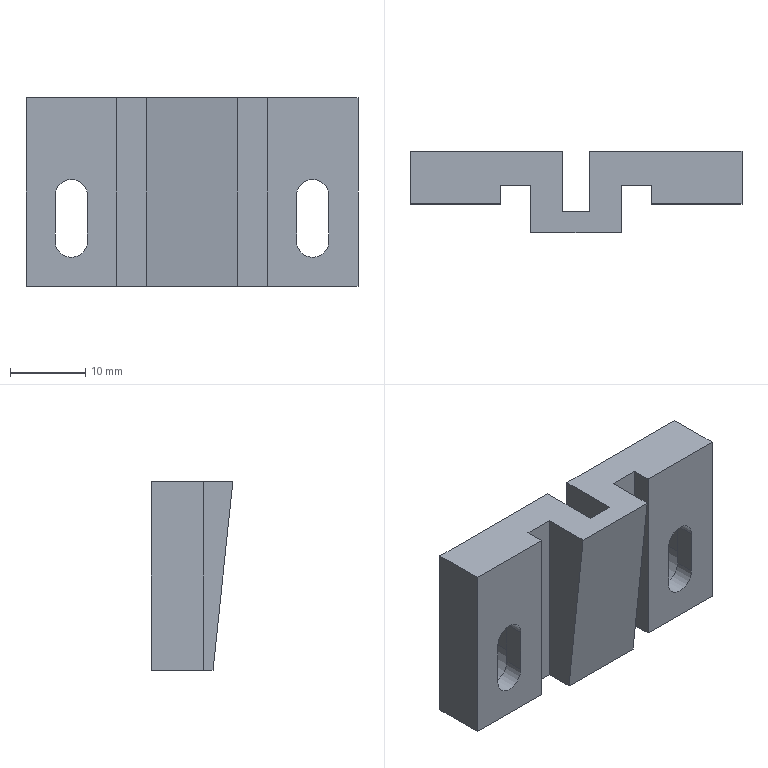Part | NX | features BREP 1 | 1 solid | 40 faces | box 44 x 10.828 x 25 mm | volume 6160 mm3 | plane 28 | cylinder 12 | commonest cylinder face diameters 4.3 x6 8 x6
STEP:
#1=CARTESIAN_POINT('',(16.,-1.,14.15));
#2=VERTEX_POINT('',#1);
#3=CARTESIAN_POINT('',(18.15,-1.,12.));
#4=VERTEX_POINT('',#3);
#5=CARTESIAN_POINT('',(16.,-1.,12.));
#6=DIRECTION('',(0.,1.,0.));
#7=DIRECTION('',(1.,0.,0.));
#8=AXIS2_PLACEMENT_3D('',#5,#6,#7);
#9=CIRCLE('',#8,2.15);
#10=EDGE_CURVE('',#2,#4,#9,.T.);
#11=ORIENTED_EDGE('',*,*,#10,.F.);
#12=CARTESIAN_POINT('',(16.,1.6,14.15));
#13=VERTEX_POINT('',#12);
#14=CARTESIAN_POINT('',(16.,-4.828,14.15));
#15=DIRECTION('',(0.,1.,0.));
#16=VECTOR('',#15,1000.);
#17=LINE('',#14,#16);
#18=EDGE_CURVE('',#2,#13,#17,.T.);
#19=ORIENTED_EDGE('',*,*,#18,.T.);
#20=CARTESIAN_POINT('',(18.15,1.6,12.));
#21=VERTEX_POINT('',#20);
#22=CARTESIAN_POINT('',(16.,1.6,12.));
#23=DIRECTION('',(0.,-1.,0.));
#24=DIRECTION('',(0.,0.,1.));
#25=AXIS2_PLACEMENT_3D('',#22,#23,#24);
#26=CIRCLE('',#25,2.15);
#27=EDGE_CURVE('',#21,#13,#26,.T.);
#28=ORIENTED_EDGE('',*,*,#27,.F.);
#29=CARTESIAN_POINT('',(18.15,-4.828,12.));
#30=DIRECTION('',(0.,1.,0.));
#31=VECTOR('',#30,1000.);
#32=LINE('',#29,#31);
#33=EDGE_CURVE('',#4,#21,#32,.T.);
#34=ORIENTED_EDGE('',*,*,#33,.F.);
#35=EDGE_LOOP('',(#11,#19,#28,#34));
#36=FACE_BOUND('',#35,.T.);
#37=CARTESIAN_POINT('',(16.,-4.828,12.));
#38=DIRECTION('',(0.,1.,0.));
#39=DIRECTION('',(0.,0.,1.));
#40=AXIS2_PLACEMENT_3D('',#37,#38,#39);
#41=CYLINDRICAL_SURFACE('',#40,2.15);
#42=ADVANCED_FACE('',(#36),#41,.F.);
#43=CARTESIAN_POINT('',(20.,1.6,12.));
#44=VERTEX_POINT('',#43);
#45=CARTESIAN_POINT('',(16.,1.6,16.));
#46=VERTEX_POINT('',#45);
#47=CARTESIAN_POINT('',(16.,1.6,12.));
#48=DIRECTION('',(0.,-1.,0.));
#49=DIRECTION('',(0.,0.,-1.));
#50=AXIS2_PLACEMENT_3D('',#47,#48,#49);
#51=CIRCLE('',#50,4.);
#52=EDGE_CURVE('',#44,#46,#51,.T.);
#53=ORIENTED_EDGE('',*,*,#52,.T.);
#54=CARTESIAN_POINT('',(16.,6.,16.));
#55=VERTEX_POINT('',#54);
#56=CARTESIAN_POINT('',(16.,-14.525,16.));
#57=DIRECTION('',(0.,1.,0.));
#58=VECTOR('',#57,1000.);
#59=LINE('',#56,#58);
#60=EDGE_CURVE('',#46,#55,#59,.T.);
#61=ORIENTED_EDGE('',*,*,#60,.T.);
#62=CARTESIAN_POINT('',(20.,6.,12.));
#63=VERTEX_POINT('',#62);
#64=CARTESIAN_POINT('',(16.,6.,12.));
#65=DIRECTION('',(0.,-1.,0.));
#66=DIRECTION('',(0.,0.,1.));
#67=AXIS2_PLACEMENT_3D('',#64,#65,#66);
#68=CIRCLE('',#67,4.);
#69=EDGE_CURVE('',#63,#55,#68,.T.);
#70=ORIENTED_EDGE('',*,*,#69,.F.);
#71=CARTESIAN_POINT('',(20.,-14.525,12.));
#72=DIRECTION('',(0.,1.,0.));
#73=VECTOR('',#72,1000.);
#74=LINE('',#71,#73);
#75=EDGE_CURVE('',#44,#63,#74,.T.);
#76=ORIENTED_EDGE('',*,*,#75,.F.);
#77=EDGE_LOOP('',(#53,#61,#70,#76));
#78=FACE_BOUND('',#77,.T.);
#79=CARTESIAN_POINT('',(16.,-14.525,12.));
#80=DIRECTION('',(0.,1.,0.));
#81=DIRECTION('',(0.,0.,1.));
#82=AXIS2_PLACEMENT_3D('',#79,#80,#81);
#83=CYLINDRICAL_SURFACE('',#82,4.);
#84=ADVANCED_FACE('',(#78),#83,.F.);
#85=CARTESIAN_POINT('',(-16.,-1.,14.15));
#86=VERTEX_POINT('',#85);
#87=CARTESIAN_POINT('',(-13.85,-1.,12.));
#88=VERTEX_POINT('',#87);
#89=CARTESIAN_POINT('',(-16.,-1.,12.));
#90=DIRECTION('',(0.,1.,0.));
#91=DIRECTION('',(-1.,0.,0.));
#92=AXIS2_PLACEMENT_3D('',#89,#90,#91);
#93=CIRCLE('',#92,2.15);
#94=EDGE_CURVE('',#86,#88,#93,.T.);
#95=ORIENTED_EDGE('',*,*,#94,.F.);
#96=CARTESIAN_POINT('',(-16.,1.6,14.15));
#97=VERTEX_POINT('',#96);
#98=CARTESIAN_POINT('',(-16.,-4.828,14.15));
#99=DIRECTION('',(0.,1.,0.));
#100=VECTOR('',#99,1000.);
#101=LINE('',#98,#100);
#102=EDGE_CURVE('',#86,#97,#101,.T.);
#103=ORIENTED_EDGE('',*,*,#102,.T.);
#104=CARTESIAN_POINT('',(-13.85,1.6,12.));
#105=VERTEX_POINT('',#104);
#106=CARTESIAN_POINT('',(-16.,1.6,12.));
#107=DIRECTION('',(0.,1.,0.));
#108=DIRECTION('',(0.,0.,1.));
#109=AXIS2_PLACEMENT_3D('',#106,#107,#108);
#110=CIRCLE('',#109,2.15);
#111=EDGE_CURVE('',#97,#105,#110,.T.);
#112=ORIENTED_EDGE('',*,*,#111,.T.);
#113=CARTESIAN_POINT('',(-13.85,-4.828,12.));
#114=DIRECTION('',(0.,1.,0.));
#115=VECTOR('',#114,1000.);
#116=LINE('',#113,#115);
#117=EDGE_CURVE('',#88,#105,#116,.T.);
#118=ORIENTED_EDGE('',*,*,#117,.F.);
#119=EDGE_LOOP('',(#95,#103,#112,#118));
#120=FACE_BOUND('',#119,.T.);
#121=CARTESIAN_POINT('',(-16.,-4.828,12.));
#122=DIRECTION('',(0.,1.,0.));
#123=DIRECTION('',(0.,0.,1.));
#124=AXIS2_PLACEMENT_3D('',#121,#122,#123);
#125=CYLINDRICAL_SURFACE('',#124,2.15);
#126=ADVANCED_FACE('',(#120),#125,.F.);
#127=CARTESIAN_POINT('',(-16.,1.6,16.));
#128=VERTEX_POINT('',#127);
#129=CARTESIAN_POINT('',(-12.,1.6,12.));
#130=VERTEX_POINT('',#129);
#131=CARTESIAN_POINT('',(-16.,1.6,12.));
#132=DIRECTION('',(0.,1.,0.));
#133=DIRECTION('',(0.,0.,-1.));
#134=AXIS2_PLACEMENT_3D('',#131,#132,#133);
#135=CIRCLE('',#134,4.);
#136=EDGE_CURVE('',#128,#130,#135,.T.);
#137=ORIENTED_EDGE('',*,*,#136,.F.);
#138=CARTESIAN_POINT('',(-16.,6.,16.));
#139=VERTEX_POINT('',#138);
#140=CARTESIAN_POINT('',(-16.,-14.525,16.));
#141=DIRECTION('',(0.,1.,0.));
#142=VECTOR('',#141,1000.);
#143=LINE('',#140,#142);
#144=EDGE_CURVE('',#128,#139,#143,.T.);
#145=ORIENTED_EDGE('',*,*,#144,.T.);
#146=CARTESIAN_POINT('',(-12.,6.,12.));
#147=VERTEX_POINT('',#146);
#148=CARTESIAN_POINT('',(-16.,6.,12.));
#149=DIRECTION('',(0.,1.,0.));
#150=DIRECTION('',(0.,0.,1.));
#151=AXIS2_PLACEMENT_3D('',#148,#149,#150);
#152=CIRCLE('',#151,4.);
#153=EDGE_CURVE('',#139,#147,#152,.T.);
#154=ORIENTED_EDGE('',*,*,#153,.T.);
#155=CARTESIAN_POINT('',(-12.,-14.525,12.));
#156=DIRECTION('',(0.,1.,0.));
#157=VECTOR('',#156,1000.);
#158=LINE('',#155,#157);
#159=EDGE_CURVE('',#130,#147,#158,.T.);
#160=ORIENTED_EDGE('',*,*,#159,.F.);
#161=EDGE_LOOP('',(#137,#145,#154,#160));
#162=FACE_BOUND('',#161,.T.);
#163=CARTESIAN_POINT('',(-16.,-14.525,12.));
#164=DIRECTION('',(0.,1.,0.));
#165=DIRECTION('',(0.,0.,1.));
#166=AXIS2_PLACEMENT_3D('',#163,#164,#165);
#167=CYLINDRICAL_SURFACE('',#166,4.);
#168=ADVANCED_FACE('',(#162),#167,.F.);
#169=CARTESIAN_POINT('',(22.,-1.,25.));
#170=VERTEX_POINT('',#169);
#171=CARTESIAN_POINT('',(10.,-1.,25.));
#172=VERTEX_POINT('',#171);
#173=CARTESIAN_POINT('',(35.634,-1.,25.));
#174=DIRECTION('',(-1.,0.,0.));
#175=VECTOR('',#174,1000.);
#176=LINE('',#173,#175);
#177=EDGE_CURVE('',#170,#172,#176,.T.);
#178=ORIENTED_EDGE('',*,*,#177,.T.);
#179=CARTESIAN_POINT('',(10.,-1.,0.));
#180=VERTEX_POINT('',#179);
#181=CARTESIAN_POINT('',(10.,-1.,25.));
#182=DIRECTION('',(0.,0.,-1.));
#183=VECTOR('',#182,1000.);
#184=LINE('',#181,#183);
#185=EDGE_CURVE('',#172,#180,#184,.T.);
#186=ORIENTED_EDGE('',*,*,#185,.T.);
#187=CARTESIAN_POINT('',(22.,-1.,0.));
#188=VERTEX_POINT('',#187);
#189=CARTESIAN_POINT('',(0.,-1.,0.));
#190=DIRECTION('',(-1.,0.,0.));
#191=VECTOR('',#190,1000.);
#192=LINE('',#189,#191);
#193=EDGE_CURVE('',#188,#180,#192,.T.);
#194=ORIENTED_EDGE('',*,*,#193,.F.);
#195=CARTESIAN_POINT('',(22.,-1.,25.));
#196=DIRECTION('',(0.,0.,1.));
#197=VECTOR('',#196,1000.);
#198=LINE('',#195,#197);
#199=EDGE_CURVE('',#188,#170,#198,.T.);
#200=ORIENTED_EDGE('',*,*,#199,.T.);
#201=EDGE_LOOP('',(#178,#186,#194,#200));
#202=FACE_BOUND('',#201,.T.);
#203=CARTESIAN_POINT('',(18.15,-1.,6.));
#204=VERTEX_POINT('',#203);
#205=CARTESIAN_POINT('',(18.15,-1.,25.));
#206=DIRECTION('',(0.,0.,-1.));
#207=VECTOR('',#206,1000.);
#208=LINE('',#205,#207);
#209=EDGE_CURVE('',#4,#204,#208,.T.);
#210=ORIENTED_EDGE('',*,*,#209,.T.);
#211=CARTESIAN_POINT('',(13.85,-1.,6.));
#212=VERTEX_POINT('',#211);
#213=CARTESIAN_POINT('',(16.,-1.,6.));
#214=DIRECTION('',(0.,1.,0.));
#215=DIRECTION('',(1.,0.,0.));
#216=AXIS2_PLACEMENT_3D('',#213,#214,#215);
#217=CIRCLE('',#216,2.15);
#218=EDGE_CURVE('',#204,#212,#217,.T.);
#219=ORIENTED_EDGE('',*,*,#218,.T.);
#220=CARTESIAN_POINT('',(13.85,-1.,12.));
#221=VERTEX_POINT('',#220);
#222=CARTESIAN_POINT('',(13.85,-1.,25.));
#223=DIRECTION('',(0.,0.,1.));
#224=VECTOR('',#223,1000.);
#225=LINE('',#222,#224);
#226=EDGE_CURVE('',#212,#221,#225,.T.);
#227=ORIENTED_EDGE('',*,*,#226,.T.);
#228=CARTESIAN_POINT('',(16.,-1.,12.));
#229=DIRECTION('',(0.,1.,0.));
#230=DIRECTION('',(1.,0.,0.));
#231=AXIS2_PLACEMENT_3D('',#228,#229,#230);
#232=CIRCLE('',#231,2.15);
#233=EDGE_CURVE('',#221,#2,#232,.T.);
#234=ORIENTED_EDGE('',*,*,#233,.T.);
#235=ORIENTED_EDGE('',*,*,#10,.T.);
#236=EDGE_LOOP('',(#210,#219,#227,#234,#235));
#237=FACE_BOUND('',#236,.T.);
#238=CARTESIAN_POINT('',(35.634,-1.,25.));
#239=DIRECTION('',(0.,-1.,0.));
#240=DIRECTION('',(0.,0.,-1.));
#241=AXIS2_PLACEMENT_3D('',#238,#239,#240);
#242=PLANE('',#241);
#243=ADVANCED_FACE('',(#202,#237),#242,.T.);
#244=CARTESIAN_POINT('',(12.,1.6,6.));
#245=VERTEX_POINT('',#244);
#246=CARTESIAN_POINT('',(20.,1.6,6.));
#247=VERTEX_POINT('',#246);
#248=CARTESIAN_POINT('',(16.,1.6,6.));
#249=DIRECTION('',(0.,-1.,0.));
#250=DIRECTION('',(0.,0.,-1.));
#251=AXIS2_PLACEMENT_3D('',#248,#249,#250);
#252=CIRCLE('',#251,4.);
#253=EDGE_CURVE('',#245,#247,#252,.T.);
#254=ORIENTED_EDGE('',*,*,#253,.F.);
#255=CARTESIAN_POINT('',(12.,1.6,12.));
#256=VERTEX_POINT('',#255);
#257=CARTESIAN_POINT('',(12.,1.6,12.));
#258=DIRECTION('',(0.,0.,-1.));
#259=VECTOR('',#258,1000.);
#260=LINE('',#257,#259);
#261=EDGE_CURVE('',#256,#245,#260,.T.);
#262=ORIENTED_EDGE('',*,*,#261,.F.);
#263=CARTESIAN_POINT('',(16.,1.6,12.));
#264=DIRECTION('',(0.,-1.,0.));
#265=DIRECTION('',(0.,0.,-1.));
#266=AXIS2_PLACEMENT_3D('',#263,#264,#265);
#267=CIRCLE('',#266,4.);
#268=EDGE_CURVE('',#46,#256,#267,.T.);
#269=ORIENTED_EDGE('',*,*,#268,.F.);
#270=ORIENTED_EDGE('',*,*,#52,.F.);
#271=CARTESIAN_POINT('',(20.,1.6,12.));
#272=DIRECTION('',(0.,0.,1.));
#273=VECTOR('',#272,1000.);
#274=LINE('',#271,#273);
#275=EDGE_CURVE('',#247,#44,#274,.T.);
#276=ORIENTED_EDGE('',*,*,#275,.F.);
#277=EDGE_LOOP('',(#254,#262,#269,#270,#276));
#278=FACE_BOUND('',#277,.T.);
#279=CARTESIAN_POINT('',(13.85,1.6,6.));
#280=VERTEX_POINT('',#279);
#281=CARTESIAN_POINT('',(18.15,1.6,6.));
#282=VERTEX_POINT('',#281);
#283=CARTESIAN_POINT('',(16.,1.6,6.));
#284=DIRECTION('',(0.,-1.,0.));
#285=DIRECTION('',(0.,0.,1.));
#286=AXIS2_PLACEMENT_3D('',#283,#284,#285);
#287=CIRCLE('',#286,2.15);
#288=EDGE_CURVE('',#280,#282,#287,.T.);
#289=ORIENTED_EDGE('',*,*,#288,.T.);
#290=CARTESIAN_POINT('',(18.15,1.6,9.));
#291=DIRECTION('',(0.,0.,-1.));
#292=VECTOR('',#291,1000.);
#293=LINE('',#290,#292);
#294=EDGE_CURVE('',#21,#282,#293,.T.);
#295=ORIENTED_EDGE('',*,*,#294,.F.);
#296=ORIENTED_EDGE('',*,*,#27,.T.);
#297=CARTESIAN_POINT('',(13.85,1.6,12.));
#298=VERTEX_POINT('',#297);
#299=CARTESIAN_POINT('',(16.,1.6,12.));
#300=DIRECTION('',(0.,-1.,0.));
#301=DIRECTION('',(0.,0.,1.));
#302=AXIS2_PLACEMENT_3D('',#299,#300,#301);
#303=CIRCLE('',#302,2.15);
#304=EDGE_CURVE('',#13,#298,#303,.T.);
#305=ORIENTED_EDGE('',*,*,#304,.T.);
#306=CARTESIAN_POINT('',(13.85,1.6,9.));
#307=DIRECTION('',(0.,0.,1.));
#308=VECTOR('',#307,1000.);
#309=LINE('',#306,#308);
#310=EDGE_CURVE('',#280,#298,#309,.T.);
#311=ORIENTED_EDGE('',*,*,#310,.F.);
#312=EDGE_LOOP('',(#289,#295,#296,#305,#311));
#313=FACE_BOUND('',#312,.T.);
#314=CARTESIAN_POINT('',(18.15,1.6,9.));
#315=DIRECTION('',(0.,-1.,0.));
#316=DIRECTION('',(0.,0.,-1.));
#317=AXIS2_PLACEMENT_3D('',#314,#315,#316);
#318=PLANE('',#317);
#319=ADVANCED_FACE('',(#278,#313),#318,.F.);
#320=CARTESIAN_POINT('',(22.,6.,0.));
#321=VERTEX_POINT('',#320);
#322=CARTESIAN_POINT('',(1.8,6.,0.));
#323=VERTEX_POINT('',#322);
#324=CARTESIAN_POINT('',(-22.,6.,0.));
#325=DIRECTION('',(-1.,0.,0.));
#326=VECTOR('',#325,1000.);
#327=LINE('',#324,#326);
#328=EDGE_CURVE('',#321,#323,#327,.T.);
#329=ORIENTED_EDGE('',*,*,#328,.T.);
#330=CARTESIAN_POINT('',(1.8,6.,25.));
#331=VERTEX_POINT('',#330);
#332=CARTESIAN_POINT('',(1.8,6.,25.));
#333=DIRECTION('',(0.,0.,1.));
#334=VECTOR('',#333,1000.);
#335=LINE('',#332,#334);
#336=EDGE_CURVE('',#323,#331,#335,.T.);
#337=ORIENTED_EDGE('',*,*,#336,.T.);
#338=CARTESIAN_POINT('',(22.,6.,25.));
#339=VERTEX_POINT('',#338);
#340=CARTESIAN_POINT('',(-22.,6.,25.));
#341=DIRECTION('',(-1.,0.,0.));
#342=VECTOR('',#341,1000.);
#343=LINE('',#340,#342);
#344=EDGE_CURVE('',#339,#331,#343,.T.);
#345=ORIENTED_EDGE('',*,*,#344,.F.);
#346=CARTESIAN_POINT('',(22.,6.,25.));
#347=DIRECTION('',(0.,0.,-1.));
#348=VECTOR('',#347,1000.);
#349=LINE('',#346,#348);
#350=EDGE_CURVE('',#339,#321,#349,.T.);
#351=ORIENTED_EDGE('',*,*,#350,.T.);
#352=EDGE_LOOP('',(#329,#337,#345,#351));
#353=FACE_BOUND('',#352,.T.);
#354=ORIENTED_EDGE('',*,*,#69,.T.);
#355=CARTESIAN_POINT('',(12.,6.,12.));
#356=VERTEX_POINT('',#355);
#357=CARTESIAN_POINT('',(16.,6.,12.));
#358=DIRECTION('',(0.,-1.,0.));
#359=DIRECTION('',(0.,0.,1.));
#360=AXIS2_PLACEMENT_3D('',#357,#358,#359);
#361=CIRCLE('',#360,4.);
#362=EDGE_CURVE('',#55,#356,#361,.T.);
#363=ORIENTED_EDGE('',*,*,#362,.T.);
#364=CARTESIAN_POINT('',(12.,6.,6.));
#365=VERTEX_POINT('',#364);
#366=CARTESIAN_POINT('',(12.,6.,12.));
#367=DIRECTION('',(0.,0.,-1.));
#368=VECTOR('',#367,1000.);
#369=LINE('',#366,#368);
#370=EDGE_CURVE('',#356,#365,#369,.T.);
#371=ORIENTED_EDGE('',*,*,#370,.T.);
#372=CARTESIAN_POINT('',(20.,6.,6.));
#373=VERTEX_POINT('',#372);
#374=CARTESIAN_POINT('',(16.,6.,6.));
#375=DIRECTION('',(0.,-1.,0.));
#376=DIRECTION('',(0.,0.,1.));
#377=AXIS2_PLACEMENT_3D('',#374,#375,#376);
#378=CIRCLE('',#377,4.);
#379=EDGE_CURVE('',#365,#373,#378,.T.);
#380=ORIENTED_EDGE('',*,*,#379,.T.);
#381=CARTESIAN_POINT('',(20.,6.,12.));
#382=DIRECTION('',(0.,0.,1.));
#383=VECTOR('',#382,1000.);
#384=LINE('',#381,#383);
#385=EDGE_CURVE('',#373,#63,#384,.T.);
#386=ORIENTED_EDGE('',*,*,#385,.T.);
#387=EDGE_LOOP('',(#354,#363,#371,#380,#386));
#388=FACE_BOUND('',#387,.T.);
#389=CARTESIAN_POINT('',(-22.,6.,25.));
#390=DIRECTION('',(0.,-1.,0.));
#391=DIRECTION('',(0.,0.,-1.));
#392=AXIS2_PLACEMENT_3D('',#389,#390,#391);
#393=PLANE('',#392);
#394=ADVANCED_FACE('',(#353,#388),#393,.F.);
#395=CARTESIAN_POINT('',(6.,1.5,25.));
#396=VERTEX_POINT('',#395);
#397=CARTESIAN_POINT('',(6.,-4.828,25.));
#398=VERTEX_POINT('',#397);
#399=CARTESIAN_POINT('',(6.,-1.,25.));
#400=DIRECTION('',(0.,-1.,0.));
#401=VECTOR('',#400,1000.);
#402=LINE('',#399,#401);
#403=EDGE_CURVE('',#396,#398,#402,.T.);
#404=ORIENTED_EDGE('',*,*,#403,.F.);
#405=CARTESIAN_POINT('',(10.,1.5,25.));
#406=VERTEX_POINT('',#405);
#407=CARTESIAN_POINT('',(6.,1.5,25.));
#408=DIRECTION('',(-1.,0.,0.));
#409=VECTOR('',#408,1000.);
#410=LINE('',#407,#409);
#411=EDGE_CURVE('',#406,#396,#410,.T.);
#412=ORIENTED_EDGE('',*,*,#411,.F.);
#413=CARTESIAN_POINT('',(10.,-1.,25.));
#414=DIRECTION('',(0.,1.,0.));
#415=VECTOR('',#414,1000.);
#416=LINE('',#413,#415);
#417=EDGE_CURVE('',#172,#406,#416,.T.);
#418=ORIENTED_EDGE('',*,*,#417,.F.);
#419=ORIENTED_EDGE('',*,*,#177,.F.);
#420=CARTESIAN_POINT('',(22.,-9.,25.));
#421=DIRECTION('',(0.,1.,0.));
#422=VECTOR('',#421,1000.);
#423=LINE('',#420,#422);
#424=EDGE_CURVE('',#170,#339,#423,.T.);
#425=ORIENTED_EDGE('',*,*,#424,.T.);
#426=ORIENTED_EDGE('',*,*,#344,.T.);
#427=CARTESIAN_POINT('',(1.8,-2.,25.));
#428=VERTEX_POINT('',#427);
#429=CARTESIAN_POINT('',(1.8,-2.2,25.));
#430=DIRECTION('',(0.,-1.,0.));
#431=VECTOR('',#430,1000.);
#432=LINE('',#429,#431);
#433=EDGE_CURVE('',#331,#428,#432,.T.);
#434=ORIENTED_EDGE('',*,*,#433,.T.);
#435=CARTESIAN_POINT('',(-1.8,-2.,25.));
#436=VERTEX_POINT('',#435);
#437=CARTESIAN_POINT('',(1.8,-2.,25.));
#438=DIRECTION('',(-1.,0.,0.));
#439=VECTOR('',#438,1000.);
#440=LINE('',#437,#439);
#441=EDGE_CURVE('',#428,#436,#440,.T.);
#442=ORIENTED_EDGE('',*,*,#441,.T.);
#443=CARTESIAN_POINT('',(-1.8,6.,25.));
#444=VERTEX_POINT('',#443);
#445=CARTESIAN_POINT('',(-1.8,-2.2,25.));
#446=DIRECTION('',(0.,1.,0.));
#447=VECTOR('',#446,1000.);
#448=LINE('',#445,#447);
#449=EDGE_CURVE('',#436,#444,#448,.T.);
#450=ORIENTED_EDGE('',*,*,#449,.T.);
#451=CARTESIAN_POINT('',(-22.,6.,25.));
#452=VERTEX_POINT('',#451);
#453=CARTESIAN_POINT('',(-22.,6.,25.));
#454=DIRECTION('',(-1.,0.,0.));
#455=VECTOR('',#454,1000.);
#456=LINE('',#453,#455);
#457=EDGE_CURVE('',#444,#452,#456,.T.);
#458=ORIENTED_EDGE('',*,*,#457,.T.);
#459=CARTESIAN_POINT('',(-22.,-1.,25.));
#460=VERTEX_POINT('',#459);
#461=CARTESIAN_POINT('',(-22.,-9.,25.));
#462=DIRECTION('',(0.,-1.,0.));
#463=VECTOR('',#462,1000.);
#464=LINE('',#461,#463);
#465=EDGE_CURVE('',#452,#460,#464,.T.);
#466=ORIENTED_EDGE('',*,*,#465,.T.);
#467=CARTESIAN_POINT('',(-10.,-1.,25.));
#468=VERTEX_POINT('',#467);
#469=CARTESIAN_POINT('',(-35.634,-1.,25.));
#470=DIRECTION('',(1.,0.,0.));
#471=VECTOR('',#470,1000.);
#472=LINE('',#469,#471);
#473=EDGE_CURVE('',#460,#468,#472,.T.);
#474=ORIENTED_EDGE('',*,*,#473,.T.);
#475=CARTESIAN_POINT('',(-10.,1.5,25.));
#476=VERTEX_POINT('',#475);
#477=CARTESIAN_POINT('',(-10.,-1.,25.));
#478=DIRECTION('',(0.,1.,0.));
#479=VECTOR('',#478,1000.);
#480=LINE('',#477,#479);
#481=EDGE_CURVE('',#468,#476,#480,.T.);
#482=ORIENTED_EDGE('',*,*,#481,.T.);
#483=CARTESIAN_POINT('',(-6.,1.5,25.));
#484=VERTEX_POINT('',#483);
#485=CARTESIAN_POINT('',(-6.,1.5,25.));
#486=DIRECTION('',(1.,0.,0.));
#487=VECTOR('',#486,1000.);
#488=LINE('',#485,#487);
#489=EDGE_CURVE('',#476,#484,#488,.T.);
#490=ORIENTED_EDGE('',*,*,#489,.T.);
#491=CARTESIAN_POINT('',(-6.,-4.828,25.));
#492=VERTEX_POINT('',#491);
#493=CARTESIAN_POINT('',(-6.,-1.,25.));
#494=DIRECTION('',(0.,-1.,0.));
#495=VECTOR('',#494,1000.);
#496=LINE('',#493,#495);
#497=EDGE_CURVE('',#484,#492,#496,.T.);
#498=ORIENTED_EDGE('',*,*,#497,.T.);
#499=CARTESIAN_POINT('',(22.,-4.828,25.));
#500=DIRECTION('',(-1.,0.,0.));
#501=VECTOR('',#500,1000.);
#502=LINE('',#499,#501);
#503=EDGE_CURVE('',#398,#492,#502,.T.);
#504=ORIENTED_EDGE('',*,*,#503,.F.);
#505=EDGE_LOOP('',(#404,#412,#418,#419,#425,#426,#434,#442,#450,#458,#466,#474,#482,#490,#498,#504));
#506=FACE_BOUND('',#505,.T.);
#507=CARTESIAN_POINT('',(0.,0.,25.));
#508=DIRECTION('',(0.,0.,-1.));
#509=DIRECTION('',(0.,-1.,0.));
#510=AXIS2_PLACEMENT_3D('',#507,#508,#509);
#511=PLANE('',#510);
#512=ADVANCED_FACE('',(#506),#511,.F.);
#513=CARTESIAN_POINT('',(10.,1.5,0.));
#514=VERTEX_POINT('',#513);
#515=CARTESIAN_POINT('',(6.,1.5,0.));
#516=VERTEX_POINT('',#515);
#517=CARTESIAN_POINT('',(6.,1.5,0.));
#518=DIRECTION('',(-1.,0.,0.));
#519=VECTOR('',#518,1000.);
#520=LINE('',#517,#519);
#521=EDGE_CURVE('',#514,#516,#520,.T.);
#522=ORIENTED_EDGE('',*,*,#521,.T.);
#523=CARTESIAN_POINT('',(6.,-2.2,0.));
#524=VERTEX_POINT('',#523);
#525=CARTESIAN_POINT('',(6.,-1.,0.));
#526=DIRECTION('',(0.,-1.,0.));
#527=VECTOR('',#526,1000.);
#528=LINE('',#525,#527);
#529=EDGE_CURVE('',#516,#524,#528,.T.);
#530=ORIENTED_EDGE('',*,*,#529,.T.);
#531=CARTESIAN_POINT('',(-6.,-2.2,0.));
#532=VERTEX_POINT('',#531);
#533=CARTESIAN_POINT('',(22.,-2.2,0.));
#534=DIRECTION('',(-1.,0.,0.));
#535=VECTOR('',#534,1000.);
#536=LINE('',#533,#535);
#537=EDGE_CURVE('',#524,#532,#536,.T.);
#538=ORIENTED_EDGE('',*,*,#537,.T.);
#539=CARTESIAN_POINT('',(-6.,1.5,0.));
#540=VERTEX_POINT('',#539);
#541=CARTESIAN_POINT('',(-6.,-1.,0.));
#542=DIRECTION('',(0.,-1.,0.));
#543=VECTOR('',#542,1000.);
#544=LINE('',#541,#543);
#545=EDGE_CURVE('',#540,#532,#544,.T.);
#546=ORIENTED_EDGE('',*,*,#545,.F.);
#547=CARTESIAN_POINT('',(-10.,1.5,0.));
#548=VERTEX_POINT('',#547);
#549=CARTESIAN_POINT('',(-6.,1.5,0.));
#550=DIRECTION('',(1.,0.,0.));
#551=VECTOR('',#550,1000.);
#552=LINE('',#549,#551);
#553=EDGE_CURVE('',#548,#540,#552,.T.);
#554=ORIENTED_EDGE('',*,*,#553,.F.);
#555=CARTESIAN_POINT('',(-10.,-1.,0.));
#556=VERTEX_POINT('',#555);
#557=CARTESIAN_POINT('',(-10.,-1.,0.));
#558=DIRECTION('',(0.,1.,0.));
#559=VECTOR('',#558,1000.);
#560=LINE('',#557,#559);
#561=EDGE_CURVE('',#556,#548,#560,.T.);
#562=ORIENTED_EDGE('',*,*,#561,.F.);
#563=CARTESIAN_POINT('',(-22.,-1.,0.));
#564=VERTEX_POINT('',#563);
#565=CARTESIAN_POINT('',(0.,-1.,0.));
#566=DIRECTION('',(1.,0.,0.));
#567=VECTOR('',#566,1000.);
#568=LINE('',#565,#567);
#569=EDGE_CURVE('',#564,#556,#568,.T.);
#570=ORIENTED_EDGE('',*,*,#569,.F.);
#571=CARTESIAN_POINT('',(-22.,6.,0.));
#572=VERTEX_POINT('',#571);
#573=CARTESIAN_POINT('',(-22.,-9.,0.));
#574=DIRECTION('',(0.,-1.,0.));
#575=VECTOR('',#574,1000.);
#576=LINE('',#573,#575);
#577=EDGE_CURVE('',#572,#564,#576,.T.);
#578=ORIENTED_EDGE('',*,*,#577,.F.);
#579=CARTESIAN_POINT('',(-1.8,6.,0.));
#580=VERTEX_POINT('',#579);
#581=CARTESIAN_POINT('',(-22.,6.,0.));
#582=DIRECTION('',(-1.,0.,0.));
#583=VECTOR('',#582,1000.);
#584=LINE('',#581,#583);
#585=EDGE_CURVE('',#580,#572,#584,.T.);
#586=ORIENTED_EDGE('',*,*,#585,.F.);
#587=CARTESIAN_POINT('',(-1.8,-2.,0.));
#588=VERTEX_POINT('',#587);
#589=CARTESIAN_POINT('',(-1.8,-2.2,0.));
#590=DIRECTION('',(0.,1.,0.));
#591=VECTOR('',#590,1000.);
#592=LINE('',#589,#591);
#593=EDGE_CURVE('',#588,#580,#592,.T.);
#594=ORIENTED_EDGE('',*,*,#593,.F.);
#595=CARTESIAN_POINT('',(1.8,-2.,0.));
#596=VERTEX_POINT('',#595);
#597=CARTESIAN_POINT('',(0.,-2.,0.));
#598=DIRECTION('',(-1.,0.,0.));
#599=VECTOR('',#598,1000.);
#600=LINE('',#597,#599);
#601=EDGE_CURVE('',#596,#588,#600,.T.);
#602=ORIENTED_EDGE('',*,*,#601,.F.);
#603=CARTESIAN_POINT('',(1.8,-2.2,0.));
#604=DIRECTION('',(0.,-1.,0.));
#605=VECTOR('',#604,1000.);
#606=LINE('',#603,#605);
#607=EDGE_CURVE('',#323,#596,#606,.T.);
#608=ORIENTED_EDGE('',*,*,#607,.F.);
#609=ORIENTED_EDGE('',*,*,#328,.F.);
#610=CARTESIAN_POINT('',(22.,-9.,0.));
#611=DIRECTION('',(0.,1.,0.));
#612=VECTOR('',#611,1000.);
#613=LINE('',#610,#612);
#614=EDGE_CURVE('',#188,#321,#613,.T.);
#615=ORIENTED_EDGE('',*,*,#614,.F.);
#616=ORIENTED_EDGE('',*,*,#193,.T.);
#617=CARTESIAN_POINT('',(10.,-1.,0.));
#618=DIRECTION('',(0.,1.,0.));
#619=VECTOR('',#618,1000.);
#620=LINE('',#617,#619);
#621=EDGE_CURVE('',#180,#514,#620,.T.);
#622=ORIENTED_EDGE('',*,*,#621,.T.);
#623=EDGE_LOOP('',(#522,#530,#538,#546,#554,#562,#570,#578,#586,#594,#602,#608,#609,#615,#616,#622));
#624=FACE_BOUND('',#623,.T.);
#625=CARTESIAN_POINT('',(0.,0.,0.));
#626=DIRECTION('',(0.,0.,-1.));
#627=DIRECTION('',(0.,-1.,0.));
#628=AXIS2_PLACEMENT_3D('',#625,#626,#627);
#629=PLANE('',#628);
#630=ADVANCED_FACE('',(#624),#629,.T.);
#631=CARTESIAN_POINT('',(-6.,-2.176,-0.2287));
#632=DIRECTION('',(0.,-0.1045,0.9945));
#633=VECTOR('',#632,1000.);
#634=LINE('',#631,#633);
#635=EDGE_CURVE('',#532,#492,#634,.T.);
#636=ORIENTED_EDGE('',*,*,#635,.T.);
#637=ORIENTED_EDGE('',*,*,#497,.F.);
#638=CARTESIAN_POINT('',(-6.,1.5,25.));
#639=DIRECTION('',(0.,0.,-1.));
#640=VECTOR('',#639,1000.);
#641=LINE('',#638,#640);
#642=EDGE_CURVE('',#484,#540,#641,.T.);
#643=ORIENTED_EDGE('',*,*,#642,.T.);
#644=ORIENTED_EDGE('',*,*,#545,.T.);
#645=EDGE_LOOP('',(#636,#637,#643,#644));
#646=FACE_BOUND('',#645,.T.);
#647=CARTESIAN_POINT('',(-6.,-1.,25.));
#648=DIRECTION('',(1.,0.,0.));
#649=DIRECTION('',(0.,1.,0.));
#650=AXIS2_PLACEMENT_3D('',#647,#648,#649);
#651=PLANE('',#650);
#652=ADVANCED_FACE('',(#646),#651,.F.);
#653=ORIENTED_EDGE('',*,*,#403,.T.);
#654=CARTESIAN_POINT('',(6.,-4.786,24.602));
#655=DIRECTION('',(0.,0.1045,-0.9945));
#656=VECTOR('',#655,1000.);
#657=LINE('',#654,#656);
#658=EDGE_CURVE('',#398,#524,#657,.T.);
#659=ORIENTED_EDGE('',*,*,#658,.T.);
#660=ORIENTED_EDGE('',*,*,#529,.F.);
#661=CARTESIAN_POINT('',(6.,1.5,25.));
#662=DIRECTION('',(0.,0.,-1.));
#663=VECTOR('',#662,1000.);
#664=LINE('',#661,#663);
#665=EDGE_CURVE('',#396,#516,#664,.T.);
#666=ORIENTED_EDGE('',*,*,#665,.F.);
#667=EDGE_LOOP('',(#653,#659,#660,#666));
#668=FACE_BOUND('',#667,.T.);
#669=CARTESIAN_POINT('',(6.,-1.,25.));
#670=DIRECTION('',(1.,0.,0.));
#671=DIRECTION('',(0.,1.,0.));
#672=AXIS2_PLACEMENT_3D('',#669,#670,#671);
#673=PLANE('',#672);
#674=ADVANCED_FACE('',(#668),#673,.T.);
#675=ORIENTED_EDGE('',*,*,#199,.F.);
#676=ORIENTED_EDGE('',*,*,#614,.T.);
#677=ORIENTED_EDGE('',*,*,#350,.F.);
#678=ORIENTED_EDGE('',*,*,#424,.F.);
#679=EDGE_LOOP('',(#675,#676,#677,#678));
#680=FACE_BOUND('',#679,.T.);
#681=CARTESIAN_POINT('',(22.,-9.,25.));
#682=DIRECTION('',(-1.,0.,0.));
#683=DIRECTION('',(0.,0.,1.));
#684=AXIS2_PLACEMENT_3D('',#681,#682,#683);
#685=PLANE('',#684);
#686=ADVANCED_FACE('',(#680),#685,.F.);
#687=ORIENTED_EDGE('',*,*,#457,.F.);
#688=CARTESIAN_POINT('',(-1.8,6.,25.));
#689=DIRECTION('',(0.,0.,-1.));
#690=VECTOR('',#689,1000.);
#691=LINE('',#688,#690);
#692=EDGE_CURVE('',#444,#580,#691,.T.);
#693=ORIENTED_EDGE('',*,*,#692,.T.);
#694=ORIENTED_EDGE('',*,*,#585,.T.);
#695=CARTESIAN_POINT('',(-22.,6.,25.));
#696=DIRECTION('',(0.,0.,-1.));
#697=VECTOR('',#696,1000.);
#698=LINE('',#695,#697);
#699=EDGE_CURVE('',#452,#572,#698,.T.);
#700=ORIENTED_EDGE('',*,*,#699,.F.);
#701=EDGE_LOOP('',(#687,#693,#694,#700));
#702=FACE_BOUND('',#701,.T.);
#703=CARTESIAN_POINT('',(-20.,6.,6.));
#704=VERTEX_POINT('',#703);
#705=CARTESIAN_POINT('',(-20.,6.,12.));
#706=VERTEX_POINT('',#705);
#707=CARTESIAN_POINT('',(-20.,6.,12.));
#708=DIRECTION('',(0.,0.,1.));
#709=VECTOR('',#708,1000.);
#710=LINE('',#707,#709);
#711=EDGE_CURVE('',#704,#706,#710,.T.);
#712=ORIENTED_EDGE('',*,*,#711,.F.);
#713=CARTESIAN_POINT('',(-12.,6.,6.));
#714=VERTEX_POINT('',#713);
#715=CARTESIAN_POINT('',(-16.,6.,6.));
#716=DIRECTION('',(0.,1.,0.));
#717=DIRECTION('',(0.,0.,1.));
#718=AXIS2_PLACEMENT_3D('',#715,#716,#717);
#719=CIRCLE('',#718,4.);
#720=EDGE_CURVE('',#714,#704,#719,.T.);
#721=ORIENTED_EDGE('',*,*,#720,.F.);
#722=CARTESIAN_POINT('',(-12.,6.,12.));
#723=DIRECTION('',(0.,0.,-1.));
#724=VECTOR('',#723,1000.);
#725=LINE('',#722,#724);
#726=EDGE_CURVE('',#147,#714,#725,.T.);
#727=ORIENTED_EDGE('',*,*,#726,.F.);
#728=ORIENTED_EDGE('',*,*,#153,.F.);
#729=CARTESIAN_POINT('',(-16.,6.,12.));
#730=DIRECTION('',(0.,1.,0.));
#731=DIRECTION('',(0.,0.,1.));
#732=AXIS2_PLACEMENT_3D('',#729,#730,#731);
#733=CIRCLE('',#732,4.);
#734=EDGE_CURVE('',#706,#139,#733,.T.);
#735=ORIENTED_EDGE('',*,*,#734,.F.);
#736=EDGE_LOOP('',(#712,#721,#727,#728,#735));
#737=FACE_BOUND('',#736,.T.);
#738=CARTESIAN_POINT('',(-22.,6.,25.));
#739=DIRECTION('',(0.,-1.,0.));
#740=DIRECTION('',(0.,0.,-1.));
#741=AXIS2_PLACEMENT_3D('',#738,#739,#740);
#742=PLANE('',#741);
#743=ADVANCED_FACE('',(#702,#737),#742,.F.);
#744=ORIENTED_EDGE('',*,*,#577,.T.);
#745=CARTESIAN_POINT('',(-22.,-1.,25.));
#746=DIRECTION('',(0.,0.,1.));
#747=VECTOR('',#746,1000.);
#748=LINE('',#745,#747);
#749=EDGE_CURVE('',#564,#460,#748,.T.);
#750=ORIENTED_EDGE('',*,*,#749,.T.);
#751=ORIENTED_EDGE('',*,*,#465,.F.);
#752=ORIENTED_EDGE('',*,*,#699,.T.);
#753=EDGE_LOOP('',(#744,#750,#751,#752));
#754=FACE_BOUND('',#753,.T.);
#755=CARTESIAN_POINT('',(-22.,-9.,25.));
#756=DIRECTION('',(1.,0.,0.));
#757=DIRECTION('',(0.,1.,0.));
#758=AXIS2_PLACEMENT_3D('',#755,#756,#757);
#759=PLANE('',#758);
#760=ADVANCED_FACE('',(#754),#759,.F.);
#761=ORIENTED_EDGE('',*,*,#569,.T.);
#762=CARTESIAN_POINT('',(-10.,-1.,25.));
#763=DIRECTION('',(0.,0.,-1.));
#764=VECTOR('',#763,1000.);
#765=LINE('',#762,#764);
#766=EDGE_CURVE('',#468,#556,#765,.T.);
#767=ORIENTED_EDGE('',*,*,#766,.F.);
#768=ORIENTED_EDGE('',*,*,#473,.F.);
#769=ORIENTED_EDGE('',*,*,#749,.F.);
#770=EDGE_LOOP('',(#761,#767,#768,#769));
#771=FACE_BOUND('',#770,.T.);
#772=CARTESIAN_POINT('',(-13.85,-1.,6.));
#773=VERTEX_POINT('',#772);
#774=CARTESIAN_POINT('',(-13.85,-1.,25.));
#775=DIRECTION('',(0.,0.,-1.));
#776=VECTOR('',#775,1000.);
#777=LINE('',#774,#776);
#778=EDGE_CURVE('',#88,#773,#777,.T.);
#779=ORIENTED_EDGE('',*,*,#778,.T.);
#780=CARTESIAN_POINT('',(-18.15,-1.,6.));
#781=VERTEX_POINT('',#780);
#782=CARTESIAN_POINT('',(-16.,-1.,6.));
#783=DIRECTION('',(0.,1.,0.));
#784=DIRECTION('',(-1.,0.,0.));
#785=AXIS2_PLACEMENT_3D('',#782,#783,#784);
#786=CIRCLE('',#785,2.15);
#787=EDGE_CURVE('',#773,#781,#786,.T.);
#788=ORIENTED_EDGE('',*,*,#787,.T.);
#789=CARTESIAN_POINT('',(-18.15,-1.,12.));
#790=VERTEX_POINT('',#789);
#791=CARTESIAN_POINT('',(-18.15,-1.,25.));
#792=DIRECTION('',(0.,0.,1.));
#793=VECTOR('',#792,1000.);
#794=LINE('',#791,#793);
#795=EDGE_CURVE('',#781,#790,#794,.T.);
#796=ORIENTED_EDGE('',*,*,#795,.T.);
#797=CARTESIAN_POINT('',(-16.,-1.,12.));
#798=DIRECTION('',(0.,1.,0.));
#799=DIRECTION('',(-1.,0.,0.));
#800=AXIS2_PLACEMENT_3D('',#797,#798,#799);
#801=CIRCLE('',#800,2.15);
#802=EDGE_CURVE('',#790,#86,#801,.T.);
#803=ORIENTED_EDGE('',*,*,#802,.T.);
#804=ORIENTED_EDGE('',*,*,#94,.T.);
#805=EDGE_LOOP('',(#779,#788,#796,#803,#804));
#806=FACE_BOUND('',#805,.T.);
#807=CARTESIAN_POINT('',(-35.634,-1.,25.));
#808=DIRECTION('',(0.,1.,0.));
#809=DIRECTION('',(1.,0.,0.));
#810=AXIS2_PLACEMENT_3D('',#807,#808,#809);
#811=PLANE('',#810);
#812=ADVANCED_FACE('',(#771,#806),#811,.F.);
#813=ORIENTED_EDGE('',*,*,#503,.T.);
#814=ORIENTED_EDGE('',*,*,#635,.F.);
#815=ORIENTED_EDGE('',*,*,#537,.F.);
#816=ORIENTED_EDGE('',*,*,#658,.F.);
#817=EDGE_LOOP('',(#813,#814,#815,#816));
#818=FACE_BOUND('',#817,.T.);
#819=CARTESIAN_POINT('',(22.,-2.176,-0.2287));
#820=DIRECTION('',(0.,-0.9945,-0.1045));
#821=DIRECTION('',(0.,0.1045,-0.9945));
#822=AXIS2_PLACEMENT_3D('',#819,#820,#821);
#823=PLANE('',#822);
#824=ADVANCED_FACE('',(#818),#823,.T.);
#825=ORIENTED_EDGE('',*,*,#607,.T.);
#826=CARTESIAN_POINT('',(1.8,-2.,25.));
#827=DIRECTION('',(0.,0.,-1.));
#828=VECTOR('',#827,1000.);
#829=LINE('',#826,#828);
#830=EDGE_CURVE('',#428,#596,#829,.T.);
#831=ORIENTED_EDGE('',*,*,#830,.F.);
#832=ORIENTED_EDGE('',*,*,#433,.F.);
#833=ORIENTED_EDGE('',*,*,#336,.F.);
#834=EDGE_LOOP('',(#825,#831,#832,#833));
#835=FACE_BOUND('',#834,.T.);
#836=CARTESIAN_POINT('',(1.8,-2.2,25.));
#837=DIRECTION('',(1.,0.,0.));
#838=DIRECTION('',(0.,-1.,0.));
#839=AXIS2_PLACEMENT_3D('',#836,#837,#838);
#840=PLANE('',#839);
#841=ADVANCED_FACE('',(#835),#840,.F.);
#842=ORIENTED_EDGE('',*,*,#449,.F.);
#843=CARTESIAN_POINT('',(-1.8,-2.,25.));
#844=DIRECTION('',(0.,0.,-1.));
#845=VECTOR('',#844,1000.);
#846=LINE('',#843,#845);
#847=EDGE_CURVE('',#436,#588,#846,.T.);
#848=ORIENTED_EDGE('',*,*,#847,.T.);
#849=ORIENTED_EDGE('',*,*,#593,.T.);
#850=ORIENTED_EDGE('',*,*,#692,.F.);
#851=EDGE_LOOP('',(#842,#848,#849,#850));
#852=FACE_BOUND('',#851,.T.);
#853=CARTESIAN_POINT('',(-1.8,-2.2,25.));
#854=DIRECTION('',(-1.,0.,0.));
#855=DIRECTION('',(0.,1.,0.));
#856=AXIS2_PLACEMENT_3D('',#853,#854,#855);
#857=PLANE('',#856);
#858=ADVANCED_FACE('',(#852),#857,.F.);
#859=ORIENTED_EDGE('',*,*,#601,.T.);
#860=ORIENTED_EDGE('',*,*,#847,.F.);
#861=ORIENTED_EDGE('',*,*,#441,.F.);
#862=ORIENTED_EDGE('',*,*,#830,.T.);
#863=EDGE_LOOP('',(#859,#860,#861,#862));
#864=FACE_BOUND('',#863,.T.);
#865=CARTESIAN_POINT('',(1.8,-2.,25.));
#866=DIRECTION('',(0.,-1.,0.));
#867=DIRECTION('',(0.,0.,-1.));
#868=AXIS2_PLACEMENT_3D('',#865,#866,#867);
#869=PLANE('',#868);
#870=ADVANCED_FACE('',(#864),#869,.F.);
#871=ORIENTED_EDGE('',*,*,#553,.T.);
#872=ORIENTED_EDGE('',*,*,#642,.F.);
#873=ORIENTED_EDGE('',*,*,#489,.F.);
#874=CARTESIAN_POINT('',(-10.,1.5,25.));
#875=DIRECTION('',(0.,0.,-1.));
#876=VECTOR('',#875,1000.);
#877=LINE('',#874,#876);
#878=EDGE_CURVE('',#476,#548,#877,.T.);
#879=ORIENTED_EDGE('',*,*,#878,.T.);
#880=EDGE_LOOP('',(#871,#872,#873,#879));
#881=FACE_BOUND('',#880,.T.);
#882=CARTESIAN_POINT('',(-6.,1.5,25.));
#883=DIRECTION('',(0.,1.,0.));
#884=DIRECTION('',(1.,0.,0.));
#885=AXIS2_PLACEMENT_3D('',#882,#883,#884);
#886=PLANE('',#885);
#887=ADVANCED_FACE('',(#881),#886,.F.);
#888=ORIENTED_EDGE('',*,*,#561,.T.);
#889=ORIENTED_EDGE('',*,*,#878,.F.);
#890=ORIENTED_EDGE('',*,*,#481,.F.);
#891=ORIENTED_EDGE('',*,*,#766,.T.);
#892=EDGE_LOOP('',(#888,#889,#890,#891));
#893=FACE_BOUND('',#892,.T.);
#894=CARTESIAN_POINT('',(-10.,-1.,25.));
#895=DIRECTION('',(-1.,0.,0.));
#896=DIRECTION('',(0.,0.,1.));
#897=AXIS2_PLACEMENT_3D('',#894,#895,#896);
#898=PLANE('',#897);
#899=ADVANCED_FACE('',(#893),#898,.F.);
#900=ORIENTED_EDGE('',*,*,#621,.F.);
#901=ORIENTED_EDGE('',*,*,#185,.F.);
#902=ORIENTED_EDGE('',*,*,#417,.T.);
#903=CARTESIAN_POINT('',(10.,1.5,25.));
#904=DIRECTION('',(0.,0.,-1.));
#905=VECTOR('',#904,1000.);
#906=LINE('',#903,#905);
#907=EDGE_CURVE('',#406,#514,#906,.T.);
#908=ORIENTED_EDGE('',*,*,#907,.T.);
#909=EDGE_LOOP('',(#900,#901,#902,#908));
#910=FACE_BOUND('',#909,.T.);
#911=CARTESIAN_POINT('',(10.,-1.,25.));
#912=DIRECTION('',(-1.,0.,0.));
#913=DIRECTION('',(0.,0.,1.));
#914=AXIS2_PLACEMENT_3D('',#911,#912,#913);
#915=PLANE('',#914);
#916=ADVANCED_FACE('',(#910),#915,.T.);
#917=ORIENTED_EDGE('',*,*,#521,.F.);
#918=ORIENTED_EDGE('',*,*,#907,.F.);
#919=ORIENTED_EDGE('',*,*,#411,.T.);
#920=ORIENTED_EDGE('',*,*,#665,.T.);
#921=EDGE_LOOP('',(#917,#918,#919,#920));
#922=FACE_BOUND('',#921,.T.);
#923=CARTESIAN_POINT('',(6.,1.5,25.));
#924=DIRECTION('',(0.,-1.,0.));
#925=DIRECTION('',(0.,0.,-1.));
#926=AXIS2_PLACEMENT_3D('',#923,#924,#925);
#927=PLANE('',#926);
#928=ADVANCED_FACE('',(#922),#927,.T.);
#929=CARTESIAN_POINT('',(-12.,1.6,6.));
#930=VERTEX_POINT('',#929);
#931=CARTESIAN_POINT('',(-20.,1.6,6.));
#932=VERTEX_POINT('',#931);
#933=CARTESIAN_POINT('',(-16.,1.6,6.));
#934=DIRECTION('',(0.,1.,0.));
#935=DIRECTION('',(0.,0.,-1.));
#936=AXIS2_PLACEMENT_3D('',#933,#934,#935);
#937=CIRCLE('',#936,4.);
#938=EDGE_CURVE('',#930,#932,#937,.T.);
#939=ORIENTED_EDGE('',*,*,#938,.T.);
#940=CARTESIAN_POINT('',(-20.,1.6,12.));
#941=VERTEX_POINT('',#940);
#942=CARTESIAN_POINT('',(-20.,1.6,12.));
#943=DIRECTION('',(0.,0.,1.));
#944=VECTOR('',#943,1000.);
#945=LINE('',#942,#944);
#946=EDGE_CURVE('',#932,#941,#945,.T.);
#947=ORIENTED_EDGE('',*,*,#946,.T.);
#948=CARTESIAN_POINT('',(-16.,1.6,12.));
#949=DIRECTION('',(0.,1.,0.));
#950=DIRECTION('',(0.,0.,-1.));
#951=AXIS2_PLACEMENT_3D('',#948,#949,#950);
#952=CIRCLE('',#951,4.);
#953=EDGE_CURVE('',#941,#128,#952,.T.);
#954=ORIENTED_EDGE('',*,*,#953,.T.);
#955=ORIENTED_EDGE('',*,*,#136,.T.);
#956=CARTESIAN_POINT('',(-12.,1.6,12.));
#957=DIRECTION('',(0.,0.,-1.));
#958=VECTOR('',#957,1000.);
#959=LINE('',#956,#958);
#960=EDGE_CURVE('',#130,#930,#959,.T.);
#961=ORIENTED_EDGE('',*,*,#960,.T.);
#962=EDGE_LOOP('',(#939,#947,#954,#955,#961));
#963=FACE_BOUND('',#962,.T.);
#964=CARTESIAN_POINT('',(-18.15,1.6,12.));
#965=VERTEX_POINT('',#964);
#966=CARTESIAN_POINT('',(-18.15,1.6,6.));
#967=VERTEX_POINT('',#966);
#968=CARTESIAN_POINT('',(-18.15,1.6,9.));
#969=DIRECTION('',(0.,0.,-1.));
#970=VECTOR('',#969,1000.);
#971=LINE('',#968,#970);
#972=EDGE_CURVE('',#965,#967,#971,.T.);
#973=ORIENTED_EDGE('',*,*,#972,.T.);
#974=CARTESIAN_POINT('',(-13.85,1.6,6.));
#975=VERTEX_POINT('',#974);
#976=CARTESIAN_POINT('',(-16.,1.6,6.));
#977=DIRECTION('',(0.,1.,0.));
#978=DIRECTION('',(0.,0.,1.));
#979=AXIS2_PLACEMENT_3D('',#976,#977,#978);
#980=CIRCLE('',#979,2.15);
#981=EDGE_CURVE('',#975,#967,#980,.T.);
#982=ORIENTED_EDGE('',*,*,#981,.F.);
#983=CARTESIAN_POINT('',(-13.85,1.6,9.));
#984=DIRECTION('',(0.,0.,1.));
#985=VECTOR('',#984,1000.);
#986=LINE('',#983,#985);
#987=EDGE_CURVE('',#975,#105,#986,.T.);
#988=ORIENTED_EDGE('',*,*,#987,.T.);
#989=ORIENTED_EDGE('',*,*,#111,.F.);
#990=CARTESIAN_POINT('',(-16.,1.6,12.));
#991=DIRECTION('',(0.,1.,0.));
#992=DIRECTION('',(0.,0.,1.));
#993=AXIS2_PLACEMENT_3D('',#990,#991,#992);
#994=CIRCLE('',#993,2.15);
#995=EDGE_CURVE('',#965,#97,#994,.T.);
#996=ORIENTED_EDGE('',*,*,#995,.F.);
#997=EDGE_LOOP('',(#973,#982,#988,#989,#996));
#998=FACE_BOUND('',#997,.T.);
#999=CARTESIAN_POINT('',(-13.85,1.6,9.));
#1000=DIRECTION('',(0.,-1.,0.));
#1001=DIRECTION('',(0.,0.,-1.));
#1002=AXIS2_PLACEMENT_3D('',#999,#1000,#1001);
#1003=PLANE('',#1002);
#1004=ADVANCED_FACE('',(#963,#998),#1003,.F.);
#1005=ORIENTED_EDGE('',*,*,#726,.T.);
#1006=CARTESIAN_POINT('',(-12.,-14.525,6.));
#1007=DIRECTION('',(0.,1.,0.));
#1008=VECTOR('',#1007,1000.);
#1009=LINE('',#1006,#1008);
#1010=EDGE_CURVE('',#930,#714,#1009,.T.);
#1011=ORIENTED_EDGE('',*,*,#1010,.F.);
#1012=ORIENTED_EDGE('',*,*,#960,.F.);
#1013=ORIENTED_EDGE('',*,*,#159,.T.);
#1014=EDGE_LOOP('',(#1005,#1011,#1012,#1013));
#1015=FACE_BOUND('',#1014,.T.);
#1016=CARTESIAN_POINT('',(-12.,-14.525,12.));
#1017=DIRECTION('',(1.,0.,0.));
#1018=DIRECTION('',(0.,0.,-1.));
#1019=AXIS2_PLACEMENT_3D('',#1016,#1017,#1018);
#1020=PLANE('',#1019);
#1021=ADVANCED_FACE('',(#1015),#1020,.F.);
#1022=ORIENTED_EDGE('',*,*,#711,.T.);
#1023=CARTESIAN_POINT('',(-20.,-14.525,12.));
#1024=DIRECTION('',(0.,1.,0.));
#1025=VECTOR('',#1024,1000.);
#1026=LINE('',#1023,#1025);
#1027=EDGE_CURVE('',#941,#706,#1026,.T.);
#1028=ORIENTED_EDGE('',*,*,#1027,.F.);
#1029=ORIENTED_EDGE('',*,*,#946,.F.);
#1030=CARTESIAN_POINT('',(-20.,-14.525,6.));
#1031=DIRECTION('',(0.,1.,0.));
#1032=VECTOR('',#1031,1000.);
#1033=LINE('',#1030,#1032);
#1034=EDGE_CURVE('',#932,#704,#1033,.T.);
#1035=ORIENTED_EDGE('',*,*,#1034,.T.);
#1036=EDGE_LOOP('',(#1022,#1028,#1029,#1035));
#1037=FACE_BOUND('',#1036,.T.);
#1038=CARTESIAN_POINT('',(-20.,-14.525,12.));
#1039=DIRECTION('',(-1.,0.,0.));
#1040=DIRECTION('',(0.,0.,1.));
#1041=AXIS2_PLACEMENT_3D('',#1038,#1039,#1040);
#1042=PLANE('',#1041);
#1043=ADVANCED_FACE('',(#1037),#1042,.F.);
#1044=ORIENTED_EDGE('',*,*,#1010,.T.);
#1045=ORIENTED_EDGE('',*,*,#720,.T.);
#1046=ORIENTED_EDGE('',*,*,#1034,.F.);
#1047=ORIENTED_EDGE('',*,*,#938,.F.);
#1048=EDGE_LOOP('',(#1044,#1045,#1046,#1047));
#1049=FACE_BOUND('',#1048,.T.);
#1050=CARTESIAN_POINT('',(-16.,-14.525,6.));
#1051=DIRECTION('',(0.,1.,0.));
#1052=DIRECTION('',(0.,0.,1.));
#1053=AXIS2_PLACEMENT_3D('',#1050,#1051,#1052);
#1054=CYLINDRICAL_SURFACE('',#1053,4.);
#1055=ADVANCED_FACE('',(#1049),#1054,.F.);
#1056=ORIENTED_EDGE('',*,*,#144,.F.);
#1057=ORIENTED_EDGE('',*,*,#953,.F.);
#1058=ORIENTED_EDGE('',*,*,#1027,.T.);
#1059=ORIENTED_EDGE('',*,*,#734,.T.);
#1060=EDGE_LOOP('',(#1056,#1057,#1058,#1059));
#1061=FACE_BOUND('',#1060,.T.);
#1062=CARTESIAN_POINT('',(-16.,-14.525,12.));
#1063=DIRECTION('',(0.,1.,0.));
#1064=DIRECTION('',(0.,0.,1.));
#1065=AXIS2_PLACEMENT_3D('',#1062,#1063,#1064);
#1066=CYLINDRICAL_SURFACE('',#1065,4.);
#1067=ADVANCED_FACE('',(#1061),#1066,.F.);
#1068=CARTESIAN_POINT('',(-13.85,-4.828,6.));
#1069=DIRECTION('',(0.,1.,0.));
#1070=VECTOR('',#1069,1000.);
#1071=LINE('',#1068,#1070);
#1072=EDGE_CURVE('',#773,#975,#1071,.T.);
#1073=ORIENTED_EDGE('',*,*,#1072,.T.);
#1074=ORIENTED_EDGE('',*,*,#981,.T.);
#1075=CARTESIAN_POINT('',(-18.15,-4.828,6.));
#1076=DIRECTION('',(0.,1.,0.));
#1077=VECTOR('',#1076,1000.);
#1078=LINE('',#1075,#1077);
#1079=EDGE_CURVE('',#781,#967,#1078,.T.);
#1080=ORIENTED_EDGE('',*,*,#1079,.F.);
#1081=ORIENTED_EDGE('',*,*,#787,.F.);
#1082=EDGE_LOOP('',(#1073,#1074,#1080,#1081));
#1083=FACE_BOUND('',#1082,.T.);
#1084=CARTESIAN_POINT('',(-16.,-4.828,6.));
#1085=DIRECTION('',(0.,1.,0.));
#1086=DIRECTION('',(0.,0.,1.));
#1087=AXIS2_PLACEMENT_3D('',#1084,#1085,#1086);
#1088=CYLINDRICAL_SURFACE('',#1087,2.15);
#1089=ADVANCED_FACE('',(#1083),#1088,.F.);
#1090=ORIENTED_EDGE('',*,*,#117,.T.);
#1091=ORIENTED_EDGE('',*,*,#987,.F.);
#1092=ORIENTED_EDGE('',*,*,#1072,.F.);
#1093=ORIENTED_EDGE('',*,*,#778,.F.);
#1094=EDGE_LOOP('',(#1090,#1091,#1092,#1093));
#1095=FACE_BOUND('',#1094,.T.);
#1096=CARTESIAN_POINT('',(-13.85,-4.828,6.));
#1097=DIRECTION('',(1.,0.,0.));
#1098=DIRECTION('',(0.,1.,0.));
#1099=AXIS2_PLACEMENT_3D('',#1096,#1097,#1098);
#1100=PLANE('',#1099);
#1101=ADVANCED_FACE('',(#1095),#1100,.F.);
#1102=ORIENTED_EDGE('',*,*,#102,.F.);
#1103=ORIENTED_EDGE('',*,*,#802,.F.);
#1104=CARTESIAN_POINT('',(-18.15,-4.828,12.));
#1105=DIRECTION('',(0.,1.,0.));
#1106=VECTOR('',#1105,1000.);
#1107=LINE('',#1104,#1106);
#1108=EDGE_CURVE('',#790,#965,#1107,.T.);
#1109=ORIENTED_EDGE('',*,*,#1108,.T.);
#1110=ORIENTED_EDGE('',*,*,#995,.T.);
#1111=EDGE_LOOP('',(#1102,#1103,#1109,#1110));
#1112=FACE_BOUND('',#1111,.T.);
#1113=CARTESIAN_POINT('',(-16.,-4.828,12.));
#1114=DIRECTION('',(0.,1.,0.));
#1115=DIRECTION('',(0.,0.,1.));
#1116=AXIS2_PLACEMENT_3D('',#1113,#1114,#1115);
#1117=CYLINDRICAL_SURFACE('',#1116,2.15);
#1118=ADVANCED_FACE('',(#1112),#1117,.F.);
#1119=ORIENTED_EDGE('',*,*,#1079,.T.);
#1120=ORIENTED_EDGE('',*,*,#972,.F.);
#1121=ORIENTED_EDGE('',*,*,#1108,.F.);
#1122=ORIENTED_EDGE('',*,*,#795,.F.);
#1123=EDGE_LOOP('',(#1119,#1120,#1121,#1122));
#1124=FACE_BOUND('',#1123,.T.);
#1125=CARTESIAN_POINT('',(-18.15,-4.828,6.));
#1126=DIRECTION('',(-1.,0.,0.));
#1127=DIRECTION('',(0.,0.,1.));
#1128=AXIS2_PLACEMENT_3D('',#1125,#1126,#1127);
#1129=PLANE('',#1128);
#1130=ADVANCED_FACE('',(#1124),#1129,.F.);
#1131=ORIENTED_EDGE('',*,*,#370,.F.);
#1132=CARTESIAN_POINT('',(12.,-14.525,12.));
#1133=DIRECTION('',(0.,1.,0.));
#1134=VECTOR('',#1133,1000.);
#1135=LINE('',#1132,#1134);
#1136=EDGE_CURVE('',#256,#356,#1135,.T.);
#1137=ORIENTED_EDGE('',*,*,#1136,.F.);
#1138=ORIENTED_EDGE('',*,*,#261,.T.);
#1139=CARTESIAN_POINT('',(12.,-14.525,6.));
#1140=DIRECTION('',(0.,1.,0.));
#1141=VECTOR('',#1140,1000.);
#1142=LINE('',#1139,#1141);
#1143=EDGE_CURVE('',#245,#365,#1142,.T.);
#1144=ORIENTED_EDGE('',*,*,#1143,.T.);
#1145=EDGE_LOOP('',(#1131,#1137,#1138,#1144));
#1146=FACE_BOUND('',#1145,.T.);
#1147=CARTESIAN_POINT('',(12.,-14.525,12.));
#1148=DIRECTION('',(1.,0.,0.));
#1149=DIRECTION('',(0.,0.,1.));
#1150=AXIS2_PLACEMENT_3D('',#1147,#1148,#1149);
#1151=PLANE('',#1150);
#1152=ADVANCED_FACE('',(#1146),#1151,.T.);
#1153=ORIENTED_EDGE('',*,*,#385,.F.);
#1154=CARTESIAN_POINT('',(20.,-14.525,6.));
#1155=DIRECTION('',(0.,1.,0.));
#1156=VECTOR('',#1155,1000.);
#1157=LINE('',#1154,#1156);
#1158=EDGE_CURVE('',#247,#373,#1157,.T.);
#1159=ORIENTED_EDGE('',*,*,#1158,.F.);
#1160=ORIENTED_EDGE('',*,*,#275,.T.);
#1161=ORIENTED_EDGE('',*,*,#75,.T.);
#1162=EDGE_LOOP('',(#1153,#1159,#1160,#1161));
#1163=FACE_BOUND('',#1162,.T.);
#1164=CARTESIAN_POINT('',(20.,-14.525,12.));
#1165=DIRECTION('',(-1.,0.,0.));
#1166=DIRECTION('',(0.,0.,1.));
#1167=AXIS2_PLACEMENT_3D('',#1164,#1165,#1166);
#1168=PLANE('',#1167);
#1169=ADVANCED_FACE('',(#1163),#1168,.T.);
#1170=ORIENTED_EDGE('',*,*,#60,.F.);
#1171=ORIENTED_EDGE('',*,*,#268,.T.);
#1172=ORIENTED_EDGE('',*,*,#1136,.T.);
#1173=ORIENTED_EDGE('',*,*,#362,.F.);
#1174=EDGE_LOOP('',(#1170,#1171,#1172,#1173));
#1175=FACE_BOUND('',#1174,.T.);
#1176=CARTESIAN_POINT('',(16.,-14.525,12.));
#1177=DIRECTION('',(0.,1.,0.));
#1178=DIRECTION('',(0.,0.,1.));
#1179=AXIS2_PLACEMENT_3D('',#1176,#1177,#1178);
#1180=CYLINDRICAL_SURFACE('',#1179,4.);
#1181=ADVANCED_FACE('',(#1175),#1180,.F.);
#1182=ORIENTED_EDGE('',*,*,#253,.T.);
#1183=ORIENTED_EDGE('',*,*,#1158,.T.);
#1184=ORIENTED_EDGE('',*,*,#379,.F.);
#1185=ORIENTED_EDGE('',*,*,#1143,.F.);
#1186=EDGE_LOOP('',(#1182,#1183,#1184,#1185));
#1187=FACE_BOUND('',#1186,.T.);
#1188=CARTESIAN_POINT('',(16.,-14.525,6.));
#1189=DIRECTION('',(0.,1.,0.));
#1190=DIRECTION('',(0.,0.,1.));
#1191=AXIS2_PLACEMENT_3D('',#1188,#1189,#1190);
#1192=CYLINDRICAL_SURFACE('',#1191,4.);
#1193=ADVANCED_FACE('',(#1187),#1192,.F.);
#1194=ORIENTED_EDGE('',*,*,#33,.T.);
#1195=ORIENTED_EDGE('',*,*,#294,.T.);
#1196=CARTESIAN_POINT('',(18.15,-4.828,6.));
#1197=DIRECTION('',(0.,1.,0.));
#1198=VECTOR('',#1197,1000.);
#1199=LINE('',#1196,#1198);
#1200=EDGE_CURVE('',#204,#282,#1199,.T.);
#1201=ORIENTED_EDGE('',*,*,#1200,.F.);
#1202=ORIENTED_EDGE('',*,*,#209,.F.);
#1203=EDGE_LOOP('',(#1194,#1195,#1201,#1202));
#1204=FACE_BOUND('',#1203,.T.);
#1205=CARTESIAN_POINT('',(18.15,-4.828,6.));
#1206=DIRECTION('',(-1.,0.,0.));
#1207=DIRECTION('',(0.,0.,1.));
#1208=AXIS2_PLACEMENT_3D('',#1205,#1206,#1207);
#1209=PLANE('',#1208);
#1210=ADVANCED_FACE('',(#1204),#1209,.T.);
#1211=CARTESIAN_POINT('',(13.85,-4.828,6.));
#1212=DIRECTION('',(0.,1.,0.));
#1213=VECTOR('',#1212,1000.);
#1214=LINE('',#1211,#1213);
#1215=EDGE_CURVE('',#212,#280,#1214,.T.);
#1216=ORIENTED_EDGE('',*,*,#1215,.T.);
#1217=ORIENTED_EDGE('',*,*,#310,.T.);
#1218=CARTESIAN_POINT('',(13.85,-4.828,12.));
#1219=DIRECTION('',(0.,1.,0.));
#1220=VECTOR('',#1219,1000.);
#1221=LINE('',#1218,#1220);
#1222=EDGE_CURVE('',#221,#298,#1221,.T.);
#1223=ORIENTED_EDGE('',*,*,#1222,.F.);
#1224=ORIENTED_EDGE('',*,*,#226,.F.);
#1225=EDGE_LOOP('',(#1216,#1217,#1223,#1224));
#1226=FACE_BOUND('',#1225,.T.);
#1227=CARTESIAN_POINT('',(13.85,-4.828,6.));
#1228=DIRECTION('',(1.,0.,0.));
#1229=DIRECTION('',(0.,1.,0.));
#1230=AXIS2_PLACEMENT_3D('',#1227,#1228,#1229);
#1231=PLANE('',#1230);
#1232=ADVANCED_FACE('',(#1226),#1231,.T.);
#1233=ORIENTED_EDGE('',*,*,#1200,.T.);
#1234=ORIENTED_EDGE('',*,*,#288,.F.);
#1235=ORIENTED_EDGE('',*,*,#1215,.F.);
#1236=ORIENTED_EDGE('',*,*,#218,.F.);
#1237=EDGE_LOOP('',(#1233,#1234,#1235,#1236));
#1238=FACE_BOUND('',#1237,.T.);
#1239=CARTESIAN_POINT('',(16.,-4.828,6.));
#1240=DIRECTION('',(0.,1.,0.));
#1241=DIRECTION('',(0.,0.,1.));
#1242=AXIS2_PLACEMENT_3D('',#1239,#1240,#1241);
#1243=CYLINDRICAL_SURFACE('',#1242,2.15);
#1244=ADVANCED_FACE('',(#1238),#1243,.F.);
#1245=ORIENTED_EDGE('',*,*,#18,.F.);
#1246=ORIENTED_EDGE('',*,*,#233,.F.);
#1247=ORIENTED_EDGE('',*,*,#1222,.T.);
#1248=ORIENTED_EDGE('',*,*,#304,.F.);
#1249=EDGE_LOOP('',(#1245,#1246,#1247,#1248));
#1250=FACE_BOUND('',#1249,.T.);
#1251=CARTESIAN_POINT('',(16.,-4.828,12.));
#1252=DIRECTION('',(0.,1.,0.));
#1253=DIRECTION('',(0.,0.,1.));
#1254=AXIS2_PLACEMENT_3D('',#1251,#1252,#1253);
#1255=CYLINDRICAL_SURFACE('',#1254,2.15);
#1256=ADVANCED_FACE('',(#1250),#1255,.F.);
#1257=CLOSED_SHELL('',(#42,#84,#126,#168,#243,#319,#394,#512,#630,#652,#674,#686,#743,#760,#812,#824,#841,#858,#870,#887,#899,#916,#928,#1004,#1021,#1043,#1055,#1067,#1089,#1101,#1118,#1130,#1152,#1169,#1181,#1193,#1210,#1232,#1244,#1256));
#1258=MANIFOLD_SOLID_BREP('',#1257);
#1259=(LENGTH_UNIT()NAMED_UNIT(*)SI_UNIT(.MILLI.,.METRE.));
#1260=UNCERTAINTY_MEASURE_WITH_UNIT(LENGTH_MEASURE(0.00001),#1259,'','');
#1261=(NAMED_UNIT(*)PLANE_ANGLE_UNIT()SI_UNIT($,.RADIAN.));
#1262=(NAMED_UNIT(*)SI_UNIT($,.STERADIAN.)SOLID_ANGLE_UNIT());
#1263=(GEOMETRIC_REPRESENTATION_CONTEXT(3)GLOBAL_UNCERTAINTY_ASSIGNED_CONTEXT((#1260))GLOBAL_UNIT_ASSIGNED_CONTEXT((#1259,#1261,#1262))REPRESENTATION_CONTEXT('',''));
#1264=ADVANCED_BREP_SHAPE_REPRESENTATION('',(#1258),#1263);